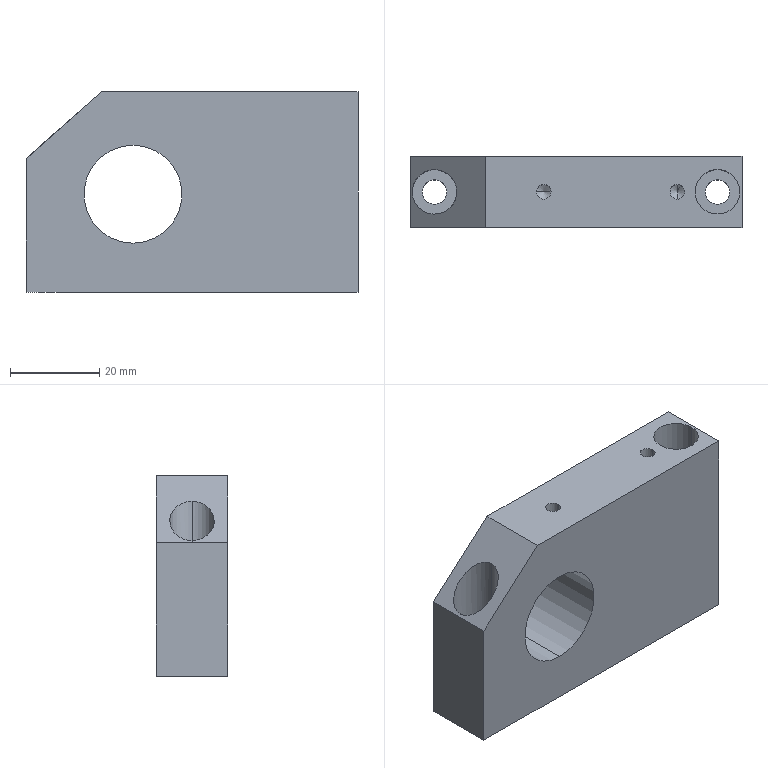Part | SolidWorks | features BaseBody 1 | 1 solid | 27 faces | box 74.5 x 16 x 45 mm | volume 40163 mm3 | cylinder 14 | plane 9 | cone 4 | commonest cylinder face diameters 3.3 x4 5.5 x4 10 x4 22 x2
STEP:
#1=CARTESIAN_POINT('',(-13.25,0.,-11.5));
#2=VERTEX_POINT('',#1);
#3=CARTESIAN_POINT('',(-13.25,0.,10.5));
#4=VERTEX_POINT('',#3);
#5=CARTESIAN_POINT('',(-13.25,0.,-0.5));
#6=DIRECTION('',(0.,1.,0.));
#7=DIRECTION('',(0.,0.,1.));
#8=AXIS2_PLACEMENT_3D('',#5,#6,#7);
#9=CIRCLE('',#8,11.);
#10=EDGE_CURVE('',#2,#4,#9,.T.);
#11=ORIENTED_EDGE('',*,*,#10,.F.);
#12=CARTESIAN_POINT('',(-13.25,16.,-11.5));
#13=VERTEX_POINT('',#12);
#14=CARTESIAN_POINT('',(-13.25,-95.,-11.5));
#15=DIRECTION('',(0.,1.,0.));
#16=VECTOR('',#15,1000.);
#17=LINE('',#14,#16);
#18=EDGE_CURVE('',#2,#13,#17,.T.);
#19=ORIENTED_EDGE('',*,*,#18,.T.);
#20=CARTESIAN_POINT('',(-13.25,16.,10.5));
#21=VERTEX_POINT('',#20);
#22=CARTESIAN_POINT('',(-13.25,16.,-0.5));
#23=DIRECTION('',(0.,-1.,0.));
#24=DIRECTION('',(0.,0.,1.));
#25=AXIS2_PLACEMENT_3D('',#22,#23,#24);
#26=CIRCLE('',#25,11.);
#27=EDGE_CURVE('',#21,#13,#26,.T.);
#28=ORIENTED_EDGE('',*,*,#27,.F.);
#29=CARTESIAN_POINT('',(-13.25,-95.,10.5));
#30=DIRECTION('',(0.,1.,0.));
#31=VECTOR('',#30,1000.);
#32=LINE('',#29,#31);
#33=EDGE_CURVE('',#4,#21,#32,.T.);
#34=ORIENTED_EDGE('',*,*,#33,.F.);
#35=EDGE_LOOP('',(#11,#19,#28,#34));
#36=FACE_OUTER_BOUND('',#35,.T.);
#37=CARTESIAN_POINT('',(-13.25,-95.,-0.5));
#38=DIRECTION('',(0.,1.,0.));
#39=DIRECTION('',(0.,0.,1.));
#40=AXIS2_PLACEMENT_3D('',#37,#38,#39);
#41=CYLINDRICAL_SURFACE('',#40,11.);
#42=ADVANCED_FACE('',(#36),#41,.F.);
#43=CARTESIAN_POINT('',(-29.,8.,-22.5));
#44=VERTEX_POINT('',#43);
#45=CARTESIAN_POINT('',(-34.5,8.,-22.5));
#46=VERTEX_POINT('',#45);
#47=CARTESIAN_POINT('',(-31.75,8.,-22.5));
#48=DIRECTION('',(0.,0.,-1.));
#49=DIRECTION('',(1.,0.,0.));
#50=AXIS2_PLACEMENT_3D('',#47,#48,#49);
#51=CIRCLE('',#50,2.75);
#52=EDGE_CURVE('',#44,#46,#51,.T.);
#53=ORIENTED_EDGE('',*,*,#52,.T.);
#54=CARTESIAN_POINT('',(-34.5,8.,-12.5));
#55=VERTEX_POINT('',#54);
#56=CARTESIAN_POINT('',(-34.5,8.,22.5));
#57=DIRECTION('',(0.,0.,1.));
#58=VECTOR('',#57,1000.);
#59=LINE('',#56,#58);
#60=EDGE_CURVE('',#46,#55,#59,.T.);
#61=ORIENTED_EDGE('',*,*,#60,.T.);
#62=CARTESIAN_POINT('',(-29.,8.,-12.5));
#63=VERTEX_POINT('',#62);
#64=CARTESIAN_POINT('',(-31.75,8.,-12.5));
#65=DIRECTION('',(0.,0.,-1.));
#66=DIRECTION('',(1.,0.,0.));
#67=AXIS2_PLACEMENT_3D('',#64,#65,#66);
#68=CIRCLE('',#67,2.75);
#69=EDGE_CURVE('',#63,#55,#68,.T.);
#70=ORIENTED_EDGE('',*,*,#69,.F.);
#71=CARTESIAN_POINT('',(-29.,8.,22.5));
#72=DIRECTION('',(0.,0.,1.));
#73=VECTOR('',#72,1000.);
#74=LINE('',#71,#73);
#75=EDGE_CURVE('',#44,#63,#74,.T.);
#76=ORIENTED_EDGE('',*,*,#75,.F.);
#77=EDGE_LOOP('',(#53,#61,#70,#76));
#78=FACE_OUTER_BOUND('',#77,.T.);
#79=CARTESIAN_POINT('',(-31.75,8.,22.5));
#80=DIRECTION('',(0.,0.,1.));
#81=DIRECTION('',(1.,0.,0.));
#82=AXIS2_PLACEMENT_3D('',#79,#80,#81);
#83=CYLINDRICAL_SURFACE('',#82,2.75);
#84=ADVANCED_FACE('',(#78),#83,.F.);
#85=CARTESIAN_POINT('',(34.5,8.,-22.5));
#86=VERTEX_POINT('',#85);
#87=CARTESIAN_POINT('',(29.,8.,-22.5));
#88=VERTEX_POINT('',#87);
#89=CARTESIAN_POINT('',(31.75,8.,-22.5));
#90=DIRECTION('',(0.,0.,-1.));
#91=DIRECTION('',(1.,0.,0.));
#92=AXIS2_PLACEMENT_3D('',#89,#90,#91);
#93=CIRCLE('',#92,2.75);
#94=EDGE_CURVE('',#86,#88,#93,.T.);
#95=ORIENTED_EDGE('',*,*,#94,.T.);
#96=CARTESIAN_POINT('',(29.,8.,-12.5));
#97=VERTEX_POINT('',#96);
#98=CARTESIAN_POINT('',(29.,8.,22.5));
#99=DIRECTION('',(0.,0.,1.));
#100=VECTOR('',#99,1000.);
#101=LINE('',#98,#100);
#102=EDGE_CURVE('',#88,#97,#101,.T.);
#103=ORIENTED_EDGE('',*,*,#102,.T.);
#104=CARTESIAN_POINT('',(34.5,8.,-12.5));
#105=VERTEX_POINT('',#104);
#106=CARTESIAN_POINT('',(31.75,8.,-12.5));
#107=DIRECTION('',(0.,0.,-1.));
#108=DIRECTION('',(1.,0.,0.));
#109=AXIS2_PLACEMENT_3D('',#106,#107,#108);
#110=CIRCLE('',#109,2.75);
#111=EDGE_CURVE('',#105,#97,#110,.T.);
#112=ORIENTED_EDGE('',*,*,#111,.F.);
#113=CARTESIAN_POINT('',(34.5,8.,22.5));
#114=DIRECTION('',(0.,0.,1.));
#115=VECTOR('',#114,1000.);
#116=LINE('',#113,#115);
#117=EDGE_CURVE('',#86,#105,#116,.T.);
#118=ORIENTED_EDGE('',*,*,#117,.F.);
#119=EDGE_LOOP('',(#95,#103,#112,#118));
#120=FACE_OUTER_BOUND('',#119,.T.);
#121=CARTESIAN_POINT('',(31.75,8.,22.5));
#122=DIRECTION('',(0.,0.,1.));
#123=DIRECTION('',(1.,0.,0.));
#124=AXIS2_PLACEMENT_3D('',#121,#122,#123);
#125=CYLINDRICAL_SURFACE('',#124,2.75);
#126=ADVANCED_FACE('',(#120),#125,.F.);
#127=CARTESIAN_POINT('',(26.75,8.,-12.5));
#128=VERTEX_POINT('',#127);
#129=CARTESIAN_POINT('',(36.75,8.,-12.5));
#130=VERTEX_POINT('',#129);
#131=CARTESIAN_POINT('',(31.75,8.,-12.5));
#132=DIRECTION('',(0.,0.,1.));
#133=DIRECTION('',(1.,0.,0.));
#134=AXIS2_PLACEMENT_3D('',#131,#132,#133);
#135=CIRCLE('',#134,5.);
#136=EDGE_CURVE('',#128,#130,#135,.T.);
#137=ORIENTED_EDGE('',*,*,#136,.F.);
#138=CARTESIAN_POINT('',(26.75,8.,22.5));
#139=VERTEX_POINT('',#138);
#140=CARTESIAN_POINT('',(26.75,8.,22.5));
#141=DIRECTION('',(0.,0.,1.));
#142=VECTOR('',#141,1000.);
#143=LINE('',#140,#142);
#144=EDGE_CURVE('',#128,#139,#143,.T.);
#145=ORIENTED_EDGE('',*,*,#144,.T.);
#146=CARTESIAN_POINT('',(36.75,8.,22.5));
#147=VERTEX_POINT('',#146);
#148=CARTESIAN_POINT('',(31.75,8.,22.5));
#149=DIRECTION('',(0.,0.,1.));
#150=DIRECTION('',(1.,0.,0.));
#151=AXIS2_PLACEMENT_3D('',#148,#149,#150);
#152=CIRCLE('',#151,5.);
#153=EDGE_CURVE('',#139,#147,#152,.T.);
#154=ORIENTED_EDGE('',*,*,#153,.T.);
#155=CARTESIAN_POINT('',(36.75,8.,22.5));
#156=DIRECTION('',(0.,0.,1.));
#157=VECTOR('',#156,1000.);
#158=LINE('',#155,#157);
#159=EDGE_CURVE('',#130,#147,#158,.T.);
#160=ORIENTED_EDGE('',*,*,#159,.F.);
#161=EDGE_LOOP('',(#137,#145,#154,#160));
#162=FACE_OUTER_BOUND('',#161,.T.);
#163=CARTESIAN_POINT('',(31.75,8.,22.5));
#164=DIRECTION('',(0.,0.,1.));
#165=DIRECTION('',(1.,0.,0.));
#166=AXIS2_PLACEMENT_3D('',#163,#164,#165);
#167=CYLINDRICAL_SURFACE('',#166,5.);
#168=ADVANCED_FACE('',(#162),#167,.F.);
#169=CARTESIAN_POINT('',(21.1,8.,12.4));
#170=VERTEX_POINT('',#169);
#171=CARTESIAN_POINT('',(22.75,6.35,12.4));
#172=VERTEX_POINT('',#171);
#173=CARTESIAN_POINT('',(22.75,8.,12.4));
#174=DIRECTION('',(0.,0.,1.));
#175=DIRECTION('',(1.,0.,0.));
#176=AXIS2_PLACEMENT_3D('',#173,#174,#175);
#177=CIRCLE('',#176,1.65);
#178=EDGE_CURVE('',#170,#172,#177,.T.);
#179=ORIENTED_EDGE('',*,*,#178,.F.);
#180=CARTESIAN_POINT('',(21.1,8.,22.5));
#181=VERTEX_POINT('',#180);
#182=CARTESIAN_POINT('',(21.1,8.,22.5));
#183=DIRECTION('',(0.,0.,1.));
#184=VECTOR('',#183,1000.);
#185=LINE('',#182,#184);
#186=EDGE_CURVE('',#170,#181,#185,.T.);
#187=ORIENTED_EDGE('',*,*,#186,.T.);
#188=CARTESIAN_POINT('',(24.4,8.,22.5));
#189=VERTEX_POINT('',#188);
#190=CARTESIAN_POINT('',(22.75,8.,22.5));
#191=DIRECTION('',(0.,0.,1.));
#192=DIRECTION('',(1.,0.,0.));
#193=AXIS2_PLACEMENT_3D('',#190,#191,#192);
#194=CIRCLE('',#193,1.65);
#195=EDGE_CURVE('',#181,#189,#194,.T.);
#196=ORIENTED_EDGE('',*,*,#195,.T.);
#197=CARTESIAN_POINT('',(24.4,8.,12.4));
#198=VERTEX_POINT('',#197);
#199=CARTESIAN_POINT('',(24.4,8.,22.5));
#200=DIRECTION('',(0.,0.,1.));
#201=VECTOR('',#200,1000.);
#202=LINE('',#199,#201);
#203=EDGE_CURVE('',#198,#189,#202,.T.);
#204=ORIENTED_EDGE('',*,*,#203,.F.);
#205=CARTESIAN_POINT('',(22.75,8.,12.4));
#206=DIRECTION('',(0.,0.,1.));
#207=DIRECTION('',(1.,0.,0.));
#208=AXIS2_PLACEMENT_3D('',#205,#206,#207);
#209=CIRCLE('',#208,1.65);
#210=EDGE_CURVE('',#172,#198,#209,.T.);
#211=ORIENTED_EDGE('',*,*,#210,.F.);
#212=EDGE_LOOP('',(#179,#187,#196,#204,#211));
#213=FACE_OUTER_BOUND('',#212,.T.);
#214=CARTESIAN_POINT('',(22.75,8.,22.5));
#215=DIRECTION('',(0.,0.,1.));
#216=DIRECTION('',(1.,0.,0.));
#217=AXIS2_PLACEMENT_3D('',#214,#215,#216);
#218=CYLINDRICAL_SURFACE('',#217,1.65);
#219=ADVANCED_FACE('',(#213),#218,.F.);
#220=CARTESIAN_POINT('',(-8.9,8.,12.4));
#221=VERTEX_POINT('',#220);
#222=CARTESIAN_POINT('',(-5.6,8.,12.4));
#223=VERTEX_POINT('',#222);
#224=CARTESIAN_POINT('',(-7.25,8.,12.4));
#225=DIRECTION('',(0.,0.,1.));
#226=DIRECTION('',(1.,0.,0.));
#227=AXIS2_PLACEMENT_3D('',#224,#225,#226);
#228=CIRCLE('',#227,1.65);
#229=EDGE_CURVE('',#221,#223,#228,.T.);
#230=ORIENTED_EDGE('',*,*,#229,.F.);
#231=CARTESIAN_POINT('',(-8.9,8.,22.5));
#232=VERTEX_POINT('',#231);
#233=CARTESIAN_POINT('',(-8.9,8.,22.5));
#234=DIRECTION('',(0.,0.,1.));
#235=VECTOR('',#234,1000.);
#236=LINE('',#233,#235);
#237=EDGE_CURVE('',#221,#232,#236,.T.);
#238=ORIENTED_EDGE('',*,*,#237,.T.);
#239=CARTESIAN_POINT('',(-5.6,8.,22.5));
#240=VERTEX_POINT('',#239);
#241=CARTESIAN_POINT('',(-7.25,8.,22.5));
#242=DIRECTION('',(0.,0.,1.));
#243=DIRECTION('',(1.,0.,0.));
#244=AXIS2_PLACEMENT_3D('',#241,#242,#243);
#245=CIRCLE('',#244,1.65);
#246=EDGE_CURVE('',#232,#240,#245,.T.);
#247=ORIENTED_EDGE('',*,*,#246,.T.);
#248=CARTESIAN_POINT('',(-5.6,8.,22.5));
#249=DIRECTION('',(0.,0.,1.));
#250=VECTOR('',#249,1000.);
#251=LINE('',#248,#250);
#252=EDGE_CURVE('',#223,#240,#251,.T.);
#253=ORIENTED_EDGE('',*,*,#252,.F.);
#254=EDGE_LOOP('',(#230,#238,#247,#253));
#255=FACE_OUTER_BOUND('',#254,.T.);
#256=CARTESIAN_POINT('',(-7.25,8.,22.5));
#257=DIRECTION('',(0.,0.,1.));
#258=DIRECTION('',(1.,0.,0.));
#259=AXIS2_PLACEMENT_3D('',#256,#257,#258);
#260=CYLINDRICAL_SURFACE('',#259,1.65);
#261=ADVANCED_FACE('',(#255),#260,.F.);
#262=CARTESIAN_POINT('',(-36.75,8.,-12.5));
#263=VERTEX_POINT('',#262);
#264=CARTESIAN_POINT('',(-26.75,8.,-12.5));
#265=VERTEX_POINT('',#264);
#266=CARTESIAN_POINT('',(-31.75,8.,-12.5));
#267=DIRECTION('',(0.,0.,1.));
#268=DIRECTION('',(1.,0.,0.));
#269=AXIS2_PLACEMENT_3D('',#266,#267,#268);
#270=CIRCLE('',#269,5.);
#271=EDGE_CURVE('',#263,#265,#270,.T.);
#272=ORIENTED_EDGE('',*,*,#271,.F.);
#273=CARTESIAN_POINT('',(-36.75,8.,7.941));
#274=VERTEX_POINT('',#273);
#275=CARTESIAN_POINT('',(-36.75,8.,22.5));
#276=DIRECTION('',(0.,0.,1.));
#277=VECTOR('',#276,1000.);
#278=LINE('',#275,#277);
#279=EDGE_CURVE('',#263,#274,#278,.T.);
#280=ORIENTED_EDGE('',*,*,#279,.T.);
#281=CARTESIAN_POINT('',(-26.75,8.,16.765));
#282=VERTEX_POINT('',#281);
#283=CARTESIAN_POINT('',(-36.75,8.,7.941));
#284=CARTESIAN_POINT('',(-36.75,-2.,7.941));
#285=CARTESIAN_POINT('',(-26.75,-2.,16.765));
#286=CARTESIAN_POINT('',(-26.75,8.,16.765));
#287=(BOUNDED_CURVE()B_SPLINE_CURVE(3,(#283,#284,#285,#286),.UNSPECIFIED.,.F.,.F.)B_SPLINE_CURVE_WITH_KNOTS((4,4),(3.142,6.283),.UNSPECIFIED.)CURVE()GEOMETRIC_REPRESENTATION_ITEM()RATIONAL_B_SPLINE_CURVE((1.,0.3333,0.3333,1.))REPRESENTATION_ITEM(''));
#288=EDGE_CURVE('',#274,#282,#287,.T.);
#289=ORIENTED_EDGE('',*,*,#288,.T.);
#290=CARTESIAN_POINT('',(-26.75,8.,22.5));
#291=DIRECTION('',(0.,0.,1.));
#292=VECTOR('',#291,1000.);
#293=LINE('',#290,#292);
#294=EDGE_CURVE('',#265,#282,#293,.T.);
#295=ORIENTED_EDGE('',*,*,#294,.F.);
#296=EDGE_LOOP('',(#272,#280,#289,#295));
#297=FACE_OUTER_BOUND('',#296,.T.);
#298=CARTESIAN_POINT('',(-31.75,8.,22.5));
#299=DIRECTION('',(0.,0.,1.));
#300=DIRECTION('',(1.,0.,0.));
#301=AXIS2_PLACEMENT_3D('',#298,#299,#300);
#302=CYLINDRICAL_SURFACE('',#301,5.);
#303=ADVANCED_FACE('',(#297),#302,.F.);
#304=CARTESIAN_POINT('',(22.75,8.,11.409));
#305=VERTEX_POINT('',#304);
#306=CARTESIAN_POINT('',(22.75,6.35,12.4));
#307=DIRECTION('',(0.,-0.8572,0.515));
#308=VECTOR('',#307,1000.);
#309=LINE('',#306,#308);
#310=EDGE_CURVE('',#305,#172,#309,.T.);
#311=ORIENTED_EDGE('',*,*,#310,.F.);
#312=CARTESIAN_POINT('',(22.75,9.65,12.4));
#313=VERTEX_POINT('',#312);
#314=CARTESIAN_POINT('',(22.75,9.65,12.4));
#315=DIRECTION('',(0.,0.8572,0.515));
#316=VECTOR('',#315,1000.);
#317=LINE('',#314,#316);
#318=EDGE_CURVE('',#305,#313,#317,.T.);
#319=ORIENTED_EDGE('',*,*,#318,.T.);
#320=CARTESIAN_POINT('',(22.75,8.,12.4));
#321=DIRECTION('',(0.,0.,1.));
#322=DIRECTION('',(1.,0.,0.));
#323=AXIS2_PLACEMENT_3D('',#320,#321,#322);
#324=CIRCLE('',#323,1.65);
#325=EDGE_CURVE('',#313,#170,#324,.T.);
#326=ORIENTED_EDGE('',*,*,#325,.T.);
#327=ORIENTED_EDGE('',*,*,#178,.T.);
#328=EDGE_LOOP('',(#311,#319,#326,#327));
#329=FACE_OUTER_BOUND('',#328,.T.);
#330=CARTESIAN_POINT('',(22.75,8.,12.4));
#331=DIRECTION('',(0.,0.,1.));
#332=DIRECTION('',(0.,-1.,0.));
#333=AXIS2_PLACEMENT_3D('',#330,#331,#332);
#334=CONICAL_SURFACE('',#333,1.65,1.03);
#335=ADVANCED_FACE('',(#329),#334,.F.);
#336=CARTESIAN_POINT('',(-7.25,8.,11.409));
#337=VERTEX_POINT('',#336);
#338=CARTESIAN_POINT('',(-5.6,8.,12.4));
#339=DIRECTION('',(0.8572,0.,0.515));
#340=VECTOR('',#339,1000.);
#341=LINE('',#338,#340);
#342=EDGE_CURVE('',#337,#223,#341,.T.);
#343=ORIENTED_EDGE('',*,*,#342,.F.);
#344=CARTESIAN_POINT('',(-8.9,8.,12.4));
#345=DIRECTION('',(-0.8572,0.,0.515));
#346=VECTOR('',#345,1000.);
#347=LINE('',#344,#346);
#348=EDGE_CURVE('',#337,#221,#347,.T.);
#349=ORIENTED_EDGE('',*,*,#348,.T.);
#350=ORIENTED_EDGE('',*,*,#229,.T.);
#351=EDGE_LOOP('',(#343,#349,#350));
#352=FACE_OUTER_BOUND('',#351,.T.);
#353=CARTESIAN_POINT('',(-7.25,8.,12.4));
#354=DIRECTION('',(0.,0.,1.));
#355=DIRECTION('',(1.,0.,0.));
#356=AXIS2_PLACEMENT_3D('',#353,#354,#355);
#357=CONICAL_SURFACE('',#356,1.65,1.03);
#358=ADVANCED_FACE('',(#352),#357,.F.);
#359=ORIENTED_EDGE('',*,*,#27,.T.);
#360=CARTESIAN_POINT('',(-13.25,16.,-0.5));
#361=DIRECTION('',(0.,-1.,0.));
#362=DIRECTION('',(0.,0.,1.));
#363=AXIS2_PLACEMENT_3D('',#360,#361,#362);
#364=CIRCLE('',#363,11.);
#365=EDGE_CURVE('',#13,#21,#364,.T.);
#366=ORIENTED_EDGE('',*,*,#365,.T.);
#367=EDGE_LOOP('',(#359,#366));
#368=FACE_BOUND('',#367,.T.);
#369=CARTESIAN_POINT('',(37.25,16.,-22.5));
#370=VERTEX_POINT('',#369);
#371=CARTESIAN_POINT('',(-37.25,16.,-22.5));
#372=VERTEX_POINT('',#371);
#373=CARTESIAN_POINT('',(0.,16.,-22.5));
#374=DIRECTION('',(-1.,0.,0.));
#375=VECTOR('',#374,1000.);
#376=LINE('',#373,#375);
#377=EDGE_CURVE('',#370,#372,#376,.T.);
#378=ORIENTED_EDGE('',*,*,#377,.T.);
#379=CARTESIAN_POINT('',(-37.25,16.,7.5));
#380=VERTEX_POINT('',#379);
#381=CARTESIAN_POINT('',(-37.25,16.,0.));
#382=DIRECTION('',(0.,0.,1.));
#383=VECTOR('',#382,1000.);
#384=LINE('',#381,#383);
#385=EDGE_CURVE('',#372,#380,#384,.T.);
#386=ORIENTED_EDGE('',*,*,#385,.T.);
#387=CARTESIAN_POINT('',(-20.25,16.,22.5));
#388=VERTEX_POINT('',#387);
#389=CARTESIAN_POINT('',(-37.25,16.,7.5));
#390=DIRECTION('',(0.7498,0.,0.6616));
#391=VECTOR('',#390,1000.);
#392=LINE('',#389,#391);
#393=EDGE_CURVE('',#380,#388,#392,.T.);
#394=ORIENTED_EDGE('',*,*,#393,.T.);
#395=CARTESIAN_POINT('',(37.25,16.,22.5));
#396=VERTEX_POINT('',#395);
#397=CARTESIAN_POINT('',(0.,16.,22.5));
#398=DIRECTION('',(1.,0.,0.));
#399=VECTOR('',#398,1000.);
#400=LINE('',#397,#399);
#401=EDGE_CURVE('',#388,#396,#400,.T.);
#402=ORIENTED_EDGE('',*,*,#401,.T.);
#403=CARTESIAN_POINT('',(37.25,16.,0.));
#404=DIRECTION('',(0.,0.,-1.));
#405=VECTOR('',#404,1000.);
#406=LINE('',#403,#405);
#407=EDGE_CURVE('',#396,#370,#406,.T.);
#408=ORIENTED_EDGE('',*,*,#407,.T.);
#409=EDGE_LOOP('',(#378,#386,#394,#402,#408));
#410=FACE_OUTER_BOUND('',#409,.T.);
#411=CARTESIAN_POINT('',(0.,16.,0.));
#412=DIRECTION('',(0.,1.,0.));
#413=DIRECTION('',(0.,0.,1.));
#414=AXIS2_PLACEMENT_3D('',#411,#412,#413);
#415=PLANE('',#414);
#416=ADVANCED_FACE('',(#368,#410),#415,.T.);
#417=ORIENTED_EDGE('',*,*,#18,.F.);
#418=CARTESIAN_POINT('',(-13.25,0.,-0.5));
#419=DIRECTION('',(0.,1.,0.));
#420=DIRECTION('',(0.,0.,1.));
#421=AXIS2_PLACEMENT_3D('',#418,#419,#420);
#422=CIRCLE('',#421,11.);
#423=EDGE_CURVE('',#4,#2,#422,.T.);
#424=ORIENTED_EDGE('',*,*,#423,.F.);
#425=ORIENTED_EDGE('',*,*,#33,.T.);
#426=ORIENTED_EDGE('',*,*,#365,.F.);
#427=EDGE_LOOP('',(#417,#424,#425,#426));
#428=FACE_OUTER_BOUND('',#427,.T.);
#429=CARTESIAN_POINT('',(-13.25,-95.,-0.5));
#430=DIRECTION('',(0.,1.,0.));
#431=DIRECTION('',(0.,0.,1.));
#432=AXIS2_PLACEMENT_3D('',#429,#430,#431);
#433=CYLINDRICAL_SURFACE('',#432,11.);
#434=ADVANCED_FACE('',(#428),#433,.F.);
#435=CARTESIAN_POINT('',(-37.25,0.,7.5));
#436=VERTEX_POINT('',#435);
#437=CARTESIAN_POINT('',(-37.25,16.,7.5));
#438=DIRECTION('',(0.,-1.,0.));
#439=VECTOR('',#438,1000.);
#440=LINE('',#437,#439);
#441=EDGE_CURVE('',#380,#436,#440,.T.);
#442=ORIENTED_EDGE('',*,*,#441,.F.);
#443=ORIENTED_EDGE('',*,*,#385,.F.);
#444=CARTESIAN_POINT('',(-37.25,0.,-22.5));
#445=VERTEX_POINT('',#444);
#446=CARTESIAN_POINT('',(-37.25,16.,-22.5));
#447=DIRECTION('',(0.,1.,0.));
#448=VECTOR('',#447,1000.);
#449=LINE('',#446,#448);
#450=EDGE_CURVE('',#445,#372,#449,.T.);
#451=ORIENTED_EDGE('',*,*,#450,.F.);
#452=CARTESIAN_POINT('',(-37.25,0.,22.5));
#453=DIRECTION('',(0.,0.,-1.));
#454=VECTOR('',#453,1000.);
#455=LINE('',#452,#454);
#456=EDGE_CURVE('',#436,#445,#455,.T.);
#457=ORIENTED_EDGE('',*,*,#456,.F.);
#458=EDGE_LOOP('',(#442,#443,#451,#457));
#459=FACE_OUTER_BOUND('',#458,.T.);
#460=CARTESIAN_POINT('',(-37.25,16.,22.5));
#461=DIRECTION('',(1.,0.,0.));
#462=DIRECTION('',(0.,0.,-1.));
#463=AXIS2_PLACEMENT_3D('',#460,#461,#462);
#464=PLANE('',#463);
#465=ADVANCED_FACE('',(#459),#464,.F.);
#466=ORIENTED_EDGE('',*,*,#450,.T.);
#467=ORIENTED_EDGE('',*,*,#377,.F.);
#468=CARTESIAN_POINT('',(37.25,0.,-22.5));
#469=VERTEX_POINT('',#468);
#470=CARTESIAN_POINT('',(37.25,16.,-22.5));
#471=DIRECTION('',(0.,1.,0.));
#472=VECTOR('',#471,1000.);
#473=LINE('',#470,#472);
#474=EDGE_CURVE('',#469,#370,#473,.T.);
#475=ORIENTED_EDGE('',*,*,#474,.F.);
#476=CARTESIAN_POINT('',(37.25,0.,-22.5));
#477=DIRECTION('',(1.,0.,0.));
#478=VECTOR('',#477,1000.);
#479=LINE('',#476,#478);
#480=EDGE_CURVE('',#445,#469,#479,.T.);
#481=ORIENTED_EDGE('',*,*,#480,.F.);
#482=EDGE_LOOP('',(#466,#467,#475,#481));
#483=FACE_OUTER_BOUND('',#482,.T.);
#484=ORIENTED_EDGE('',*,*,#52,.F.);
#485=CARTESIAN_POINT('',(-31.75,8.,-22.5));
#486=DIRECTION('',(0.,0.,-1.));
#487=DIRECTION('',(1.,0.,0.));
#488=AXIS2_PLACEMENT_3D('',#485,#486,#487);
#489=CIRCLE('',#488,2.75);
#490=EDGE_CURVE('',#46,#44,#489,.T.);
#491=ORIENTED_EDGE('',*,*,#490,.F.);
#492=EDGE_LOOP('',(#484,#491));
#493=FACE_BOUND('',#492,.T.);
#494=ORIENTED_EDGE('',*,*,#94,.F.);
#495=CARTESIAN_POINT('',(31.75,8.,-22.5));
#496=DIRECTION('',(0.,0.,-1.));
#497=DIRECTION('',(1.,0.,0.));
#498=AXIS2_PLACEMENT_3D('',#495,#496,#497);
#499=CIRCLE('',#498,2.75);
#500=EDGE_CURVE('',#88,#86,#499,.T.);
#501=ORIENTED_EDGE('',*,*,#500,.F.);
#502=EDGE_LOOP('',(#494,#501));
#503=FACE_BOUND('',#502,.T.);
#504=CARTESIAN_POINT('',(37.25,16.,-22.5));
#505=DIRECTION('',(0.,0.,1.));
#506=DIRECTION('',(1.,0.,0.));
#507=AXIS2_PLACEMENT_3D('',#504,#505,#506);
#508=PLANE('',#507);
#509=ADVANCED_FACE('',(#483,#493,#503),#508,.F.);
#510=ORIENTED_EDGE('',*,*,#474,.T.);
#511=ORIENTED_EDGE('',*,*,#407,.F.);
#512=CARTESIAN_POINT('',(37.25,0.,22.5));
#513=VERTEX_POINT('',#512);
#514=CARTESIAN_POINT('',(37.25,16.,22.5));
#515=DIRECTION('',(0.,1.,0.));
#516=VECTOR('',#515,1000.);
#517=LINE('',#514,#516);
#518=EDGE_CURVE('',#513,#396,#517,.T.);
#519=ORIENTED_EDGE('',*,*,#518,.F.);
#520=CARTESIAN_POINT('',(37.25,0.,22.5));
#521=DIRECTION('',(0.,0.,1.));
#522=VECTOR('',#521,1000.);
#523=LINE('',#520,#522);
#524=EDGE_CURVE('',#469,#513,#523,.T.);
#525=ORIENTED_EDGE('',*,*,#524,.F.);
#526=EDGE_LOOP('',(#510,#511,#519,#525));
#527=FACE_OUTER_BOUND('',#526,.T.);
#528=CARTESIAN_POINT('',(37.25,16.,22.5));
#529=DIRECTION('',(-1.,0.,0.));
#530=DIRECTION('',(0.,0.,1.));
#531=AXIS2_PLACEMENT_3D('',#528,#529,#530);
#532=PLANE('',#531);
#533=ADVANCED_FACE('',(#527),#532,.F.);
#534=CARTESIAN_POINT('',(-20.25,0.,22.5));
#535=VERTEX_POINT('',#534);
#536=CARTESIAN_POINT('',(-20.25,16.,22.5));
#537=DIRECTION('',(0.,1.,0.));
#538=VECTOR('',#537,1000.);
#539=LINE('',#536,#538);
#540=EDGE_CURVE('',#535,#388,#539,.T.);
#541=ORIENTED_EDGE('',*,*,#540,.F.);
#542=CARTESIAN_POINT('',(37.25,0.,22.5));
#543=DIRECTION('',(-1.,0.,0.));
#544=VECTOR('',#543,1000.);
#545=LINE('',#542,#544);
#546=EDGE_CURVE('',#513,#535,#545,.T.);
#547=ORIENTED_EDGE('',*,*,#546,.F.);
#548=ORIENTED_EDGE('',*,*,#518,.T.);
#549=ORIENTED_EDGE('',*,*,#401,.F.);
#550=EDGE_LOOP('',(#541,#547,#548,#549));
#551=FACE_OUTER_BOUND('',#550,.T.);
#552=CARTESIAN_POINT('',(31.75,8.,22.5));
#553=DIRECTION('',(0.,0.,1.));
#554=DIRECTION('',(1.,0.,0.));
#555=AXIS2_PLACEMENT_3D('',#552,#553,#554);
#556=CIRCLE('',#555,5.);
#557=EDGE_CURVE('',#147,#139,#556,.T.);
#558=ORIENTED_EDGE('',*,*,#557,.F.);
#559=ORIENTED_EDGE('',*,*,#153,.F.);
#560=EDGE_LOOP('',(#558,#559));
#561=FACE_BOUND('',#560,.T.);
#562=CARTESIAN_POINT('',(22.75,8.,22.5));
#563=DIRECTION('',(0.,0.,1.));
#564=DIRECTION('',(1.,0.,0.));
#565=AXIS2_PLACEMENT_3D('',#562,#563,#564);
#566=CIRCLE('',#565,1.65);
#567=EDGE_CURVE('',#189,#181,#566,.T.);
#568=ORIENTED_EDGE('',*,*,#567,.F.);
#569=ORIENTED_EDGE('',*,*,#195,.F.);
#570=EDGE_LOOP('',(#568,#569));
#571=FACE_BOUND('',#570,.T.);
#572=CARTESIAN_POINT('',(-7.25,8.,22.5));
#573=DIRECTION('',(0.,0.,1.));
#574=DIRECTION('',(1.,0.,0.));
#575=AXIS2_PLACEMENT_3D('',#572,#573,#574);
#576=CIRCLE('',#575,1.65);
#577=EDGE_CURVE('',#240,#232,#576,.T.);
#578=ORIENTED_EDGE('',*,*,#577,.F.);
#579=ORIENTED_EDGE('',*,*,#246,.F.);
#580=EDGE_LOOP('',(#578,#579));
#581=FACE_BOUND('',#580,.T.);
#582=CARTESIAN_POINT('',(37.25,16.,22.5));
#583=DIRECTION('',(0.,0.,-1.));
#584=DIRECTION('',(-1.,0.,0.));
#585=AXIS2_PLACEMENT_3D('',#582,#583,#584);
#586=PLANE('',#585);
#587=ADVANCED_FACE('',(#551,#561,#571,#581),#586,.F.);
#588=ORIENTED_EDGE('',*,*,#441,.T.);
#589=CARTESIAN_POINT('',(-20.25,0.,22.5));
#590=DIRECTION('',(-0.7498,0.,-0.6616));
#591=VECTOR('',#590,1000.);
#592=LINE('',#589,#591);
#593=EDGE_CURVE('',#535,#436,#592,.T.);
#594=ORIENTED_EDGE('',*,*,#593,.F.);
#595=ORIENTED_EDGE('',*,*,#540,.T.);
#596=ORIENTED_EDGE('',*,*,#393,.F.);
#597=EDGE_LOOP('',(#588,#594,#595,#596));
#598=FACE_OUTER_BOUND('',#597,.T.);
#599=CARTESIAN_POINT('',(-26.75,8.,16.765));
#600=CARTESIAN_POINT('',(-26.75,18.,16.765));
#601=CARTESIAN_POINT('',(-36.75,18.,7.941));
#602=CARTESIAN_POINT('',(-36.75,8.,7.941));
#603=(BOUNDED_CURVE()B_SPLINE_CURVE(3,(#599,#600,#601,#602),.UNSPECIFIED.,.F.,.F.)B_SPLINE_CURVE_WITH_KNOTS((4,4),(0.,3.142),.UNSPECIFIED.)CURVE()GEOMETRIC_REPRESENTATION_ITEM()RATIONAL_B_SPLINE_CURVE((1.,0.3333,0.3333,1.))REPRESENTATION_ITEM(''));
#604=EDGE_CURVE('',#282,#274,#603,.T.);
#605=ORIENTED_EDGE('',*,*,#604,.F.);
#606=ORIENTED_EDGE('',*,*,#288,.F.);
#607=EDGE_LOOP('',(#605,#606));
#608=FACE_BOUND('',#607,.T.);
#609=CARTESIAN_POINT('',(-20.25,35.,22.5));
#610=DIRECTION('',(0.6616,0.,-0.7498));
#611=DIRECTION('',(-0.7498,0.,-0.6616));
#612=AXIS2_PLACEMENT_3D('',#609,#610,#611);
#613=PLANE('',#612);
#614=ADVANCED_FACE('',(#598,#608),#613,.F.);
#615=ORIENTED_EDGE('',*,*,#593,.T.);
#616=ORIENTED_EDGE('',*,*,#456,.T.);
#617=ORIENTED_EDGE('',*,*,#480,.T.);
#618=ORIENTED_EDGE('',*,*,#524,.T.);
#619=ORIENTED_EDGE('',*,*,#546,.T.);
#620=EDGE_LOOP('',(#615,#616,#617,#618,#619));
#621=FACE_OUTER_BOUND('',#620,.T.);
#622=ORIENTED_EDGE('',*,*,#423,.T.);
#623=ORIENTED_EDGE('',*,*,#10,.T.);
#624=EDGE_LOOP('',(#622,#623));
#625=FACE_BOUND('',#624,.T.);
#626=CARTESIAN_POINT('',(0.,0.,0.));
#627=DIRECTION('',(0.,1.,0.));
#628=DIRECTION('',(0.,0.,1.));
#629=AXIS2_PLACEMENT_3D('',#626,#627,#628);
#630=PLANE('',#629);
#631=ADVANCED_FACE('',(#621,#625),#630,.F.);
#632=ORIENTED_EDGE('',*,*,#60,.F.);
#633=ORIENTED_EDGE('',*,*,#490,.T.);
#634=ORIENTED_EDGE('',*,*,#75,.T.);
#635=CARTESIAN_POINT('',(-31.75,8.,-12.5));
#636=DIRECTION('',(0.,0.,-1.));
#637=DIRECTION('',(1.,0.,0.));
#638=AXIS2_PLACEMENT_3D('',#635,#636,#637);
#639=CIRCLE('',#638,2.75);
#640=EDGE_CURVE('',#55,#63,#639,.T.);
#641=ORIENTED_EDGE('',*,*,#640,.F.);
#642=EDGE_LOOP('',(#632,#633,#634,#641));
#643=FACE_OUTER_BOUND('',#642,.T.);
#644=CARTESIAN_POINT('',(-31.75,8.,22.5));
#645=DIRECTION('',(0.,0.,1.));
#646=DIRECTION('',(1.,0.,0.));
#647=AXIS2_PLACEMENT_3D('',#644,#645,#646);
#648=CYLINDRICAL_SURFACE('',#647,2.75);
#649=ADVANCED_FACE('',(#643),#648,.F.);
#650=ORIENTED_EDGE('',*,*,#102,.F.);
#651=ORIENTED_EDGE('',*,*,#500,.T.);
#652=ORIENTED_EDGE('',*,*,#117,.T.);
#653=CARTESIAN_POINT('',(31.75,8.,-12.5));
#654=DIRECTION('',(0.,0.,-1.));
#655=DIRECTION('',(1.,0.,0.));
#656=AXIS2_PLACEMENT_3D('',#653,#654,#655);
#657=CIRCLE('',#656,2.75);
#658=EDGE_CURVE('',#97,#105,#657,.T.);
#659=ORIENTED_EDGE('',*,*,#658,.F.);
#660=EDGE_LOOP('',(#650,#651,#652,#659));
#661=FACE_OUTER_BOUND('',#660,.T.);
#662=CARTESIAN_POINT('',(31.75,8.,22.5));
#663=DIRECTION('',(0.,0.,1.));
#664=DIRECTION('',(1.,0.,0.));
#665=AXIS2_PLACEMENT_3D('',#662,#663,#664);
#666=CYLINDRICAL_SURFACE('',#665,2.75);
#667=ADVANCED_FACE('',(#661),#666,.F.);
#668=ORIENTED_EDGE('',*,*,#144,.F.);
#669=CARTESIAN_POINT('',(31.75,8.,-12.5));
#670=DIRECTION('',(0.,0.,1.));
#671=DIRECTION('',(1.,0.,0.));
#672=AXIS2_PLACEMENT_3D('',#669,#670,#671);
#673=CIRCLE('',#672,5.);
#674=EDGE_CURVE('',#130,#128,#673,.T.);
#675=ORIENTED_EDGE('',*,*,#674,.F.);
#676=ORIENTED_EDGE('',*,*,#159,.T.);
#677=ORIENTED_EDGE('',*,*,#557,.T.);
#678=EDGE_LOOP('',(#668,#675,#676,#677));
#679=FACE_OUTER_BOUND('',#678,.T.);
#680=CARTESIAN_POINT('',(31.75,8.,22.5));
#681=DIRECTION('',(0.,0.,1.));
#682=DIRECTION('',(1.,0.,0.));
#683=AXIS2_PLACEMENT_3D('',#680,#681,#682);
#684=CYLINDRICAL_SURFACE('',#683,5.);
#685=ADVANCED_FACE('',(#679),#684,.F.);
#686=ORIENTED_EDGE('',*,*,#186,.F.);
#687=ORIENTED_EDGE('',*,*,#325,.F.);
#688=CARTESIAN_POINT('',(22.75,8.,12.4));
#689=DIRECTION('',(0.,0.,1.));
#690=DIRECTION('',(1.,0.,0.));
#691=AXIS2_PLACEMENT_3D('',#688,#689,#690);
#692=CIRCLE('',#691,1.65);
#693=EDGE_CURVE('',#198,#313,#692,.T.);
#694=ORIENTED_EDGE('',*,*,#693,.F.);
#695=ORIENTED_EDGE('',*,*,#203,.T.);
#696=ORIENTED_EDGE('',*,*,#567,.T.);
#697=EDGE_LOOP('',(#686,#687,#694,#695,#696));
#698=FACE_OUTER_BOUND('',#697,.T.);
#699=CARTESIAN_POINT('',(22.75,8.,22.5));
#700=DIRECTION('',(0.,0.,1.));
#701=DIRECTION('',(1.,0.,0.));
#702=AXIS2_PLACEMENT_3D('',#699,#700,#701);
#703=CYLINDRICAL_SURFACE('',#702,1.65);
#704=ADVANCED_FACE('',(#698),#703,.F.);
#705=ORIENTED_EDGE('',*,*,#237,.F.);
#706=CARTESIAN_POINT('',(-7.25,8.,12.4));
#707=DIRECTION('',(0.,0.,1.));
#708=DIRECTION('',(1.,0.,0.));
#709=AXIS2_PLACEMENT_3D('',#706,#707,#708);
#710=CIRCLE('',#709,1.65);
#711=EDGE_CURVE('',#223,#221,#710,.T.);
#712=ORIENTED_EDGE('',*,*,#711,.F.);
#713=ORIENTED_EDGE('',*,*,#252,.T.);
#714=ORIENTED_EDGE('',*,*,#577,.T.);
#715=EDGE_LOOP('',(#705,#712,#713,#714));
#716=FACE_OUTER_BOUND('',#715,.T.);
#717=CARTESIAN_POINT('',(-7.25,8.,22.5));
#718=DIRECTION('',(0.,0.,1.));
#719=DIRECTION('',(1.,0.,0.));
#720=AXIS2_PLACEMENT_3D('',#717,#718,#719);
#721=CYLINDRICAL_SURFACE('',#720,1.65);
#722=ADVANCED_FACE('',(#716),#721,.F.);
#723=ORIENTED_EDGE('',*,*,#279,.F.);
#724=CARTESIAN_POINT('',(-31.75,8.,-12.5));
#725=DIRECTION('',(0.,0.,1.));
#726=DIRECTION('',(1.,0.,0.));
#727=AXIS2_PLACEMENT_3D('',#724,#725,#726);
#728=CIRCLE('',#727,5.);
#729=EDGE_CURVE('',#265,#263,#728,.T.);
#730=ORIENTED_EDGE('',*,*,#729,.F.);
#731=ORIENTED_EDGE('',*,*,#294,.T.);
#732=ORIENTED_EDGE('',*,*,#604,.T.);
#733=EDGE_LOOP('',(#723,#730,#731,#732));
#734=FACE_OUTER_BOUND('',#733,.T.);
#735=CARTESIAN_POINT('',(-31.75,8.,22.5));
#736=DIRECTION('',(0.,0.,1.));
#737=DIRECTION('',(1.,0.,0.));
#738=AXIS2_PLACEMENT_3D('',#735,#736,#737);
#739=CYLINDRICAL_SURFACE('',#738,5.);
#740=ADVANCED_FACE('',(#734),#739,.F.);
#741=ORIENTED_EDGE('',*,*,#729,.T.);
#742=ORIENTED_EDGE('',*,*,#271,.T.);
#743=EDGE_LOOP('',(#741,#742));
#744=FACE_OUTER_BOUND('',#743,.T.);
#745=ORIENTED_EDGE('',*,*,#69,.T.);
#746=ORIENTED_EDGE('',*,*,#640,.T.);
#747=EDGE_LOOP('',(#745,#746));
#748=FACE_BOUND('',#747,.T.);
#749=CARTESIAN_POINT('',(-29.,8.,-12.5));
#750=DIRECTION('',(0.,0.,-1.));
#751=DIRECTION('',(-1.,0.,0.));
#752=AXIS2_PLACEMENT_3D('',#749,#750,#751);
#753=PLANE('',#752);
#754=ADVANCED_FACE('',(#744,#748),#753,.F.);
#755=ORIENTED_EDGE('',*,*,#674,.T.);
#756=ORIENTED_EDGE('',*,*,#136,.T.);
#757=EDGE_LOOP('',(#755,#756));
#758=FACE_OUTER_BOUND('',#757,.T.);
#759=ORIENTED_EDGE('',*,*,#111,.T.);
#760=ORIENTED_EDGE('',*,*,#658,.T.);
#761=EDGE_LOOP('',(#759,#760));
#762=FACE_BOUND('',#761,.T.);
#763=CARTESIAN_POINT('',(34.5,8.,-12.5));
#764=DIRECTION('',(0.,0.,-1.));
#765=DIRECTION('',(-1.,0.,0.));
#766=AXIS2_PLACEMENT_3D('',#763,#764,#765);
#767=PLANE('',#766);
#768=ADVANCED_FACE('',(#758,#762),#767,.F.);
#769=ORIENTED_EDGE('',*,*,#318,.F.);
#770=ORIENTED_EDGE('',*,*,#310,.T.);
#771=ORIENTED_EDGE('',*,*,#210,.T.);
#772=ORIENTED_EDGE('',*,*,#693,.T.);
#773=EDGE_LOOP('',(#769,#770,#771,#772));
#774=FACE_OUTER_BOUND('',#773,.T.);
#775=CARTESIAN_POINT('',(22.75,8.,12.4));
#776=DIRECTION('',(0.,0.,1.));
#777=DIRECTION('',(0.,-1.,0.));
#778=AXIS2_PLACEMENT_3D('',#775,#776,#777);
#779=CONICAL_SURFACE('',#778,1.65,1.03);
#780=ADVANCED_FACE('',(#774),#779,.F.);
#781=ORIENTED_EDGE('',*,*,#348,.F.);
#782=ORIENTED_EDGE('',*,*,#342,.T.);
#783=ORIENTED_EDGE('',*,*,#711,.T.);
#784=EDGE_LOOP('',(#781,#782,#783));
#785=FACE_OUTER_BOUND('',#784,.T.);
#786=CARTESIAN_POINT('',(-7.25,8.,12.4));
#787=DIRECTION('',(0.,0.,1.));
#788=DIRECTION('',(1.,0.,0.));
#789=AXIS2_PLACEMENT_3D('',#786,#787,#788);
#790=CONICAL_SURFACE('',#789,1.65,1.03);
#791=ADVANCED_FACE('',(#785),#790,.F.);
#792=CLOSED_SHELL('',(#42,#84,#126,#168,#219,#261,#303,#335,#358,#416,#434,#465,#509,#533,#587,#614,#631,#649,#667,#685,#704,#722,#740,#754,#768,#780,#791));
#793=MANIFOLD_SOLID_BREP('',#792);
#794=CARTESIAN_POINT('',(0.,0.,0.));
#795=DIRECTION('',(0.,0.,1.));
#796=DIRECTION('',(1.,0.,0.));
#797=AXIS2_PLACEMENT_3D('',#794,#795,#796);
#798=(LENGTH_UNIT()NAMED_UNIT(*)SI_UNIT(.MILLI.,.METRE.));
#799=UNCERTAINTY_MEASURE_WITH_UNIT(LENGTH_MEASURE(0.00001),#798,'','');
#800=(NAMED_UNIT(*)PLANE_ANGLE_UNIT()SI_UNIT($,.RADIAN.));
#801=(NAMED_UNIT(*)SI_UNIT($,.STERADIAN.)SOLID_ANGLE_UNIT());
#802=(GEOMETRIC_REPRESENTATION_CONTEXT(3)GLOBAL_UNCERTAINTY_ASSIGNED_CONTEXT((#799))GLOBAL_UNIT_ASSIGNED_CONTEXT((#798,#800,#801))REPRESENTATION_CONTEXT('',''));
#803=ADVANCED_BREP_SHAPE_REPRESENTATION('',(#793,#797),#802);